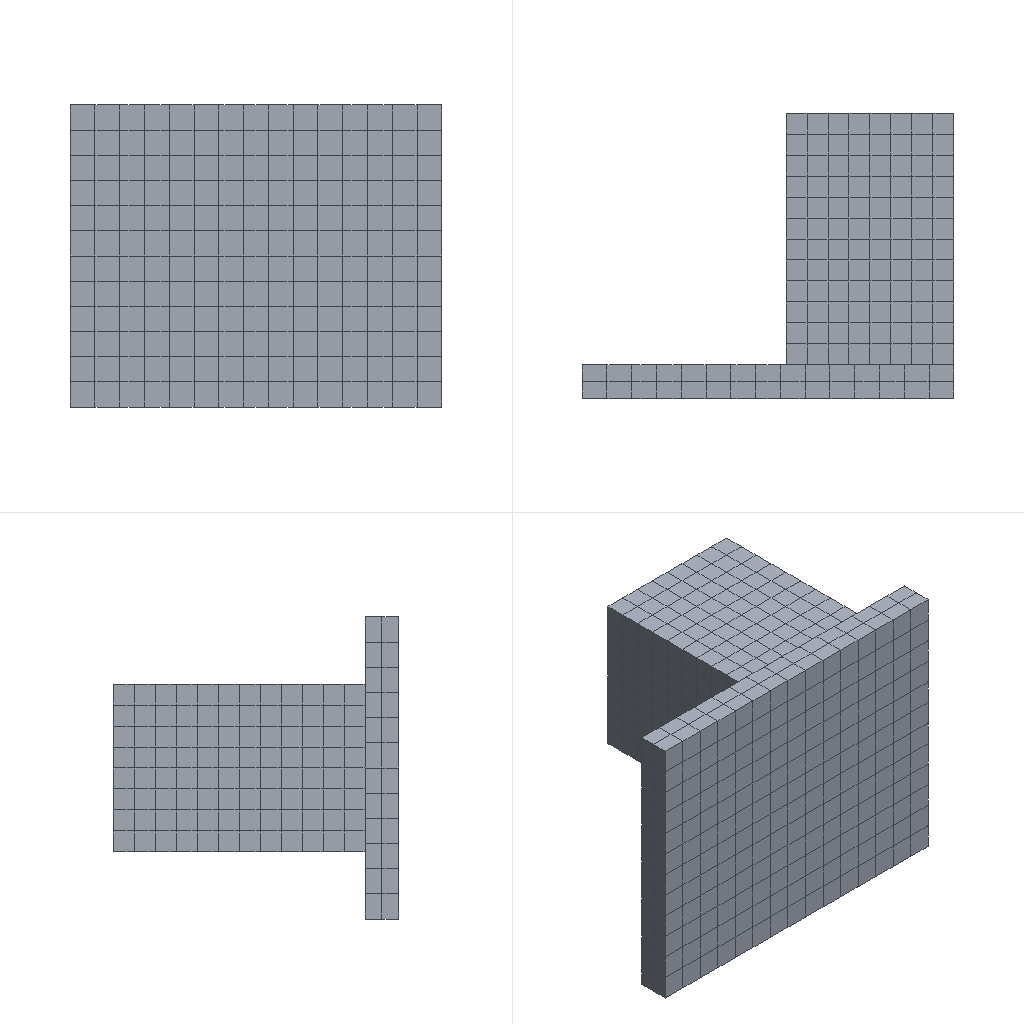Simulation study | ansys workbench
Ansys APDL input file, long lists of numbers shortened:
/batch
/config,noeldb,1     ! force off writing results to database
*get,_wallstrt,active,,time,wall
! ANSYS input file written by Workbench version 2022 R1
! File used for geometry attach:
/title,wbnew--____ (B5)
! ****** Begin Custom Load Command Snippet ******
/COM, ACT Extensions:
/COM,     LSDYNA, 2021.1
/COM,
! ****** End   Custom Load Command Snippet ******
*DIM,_wb_ProjectScratch_dir,string,248
_wb_ProjectScratch_dir(1) = ''
*DIM,_wb_SolverFiles_dir,string,248
_wb_SolverFiles_dir(1) = ''
*DIM,_wb_userfiles_dir,string,248
_wb_userfiles_dir(1) = ''
/com,--- Data in consistent NMM units. See Solving Units in the help system for more information.
/units,MPA
/nopr
/wb,file,start              !  signify a WB generated input file
/prep7
! Turn off shape checking because checks already performed inside WB mesher.
! See help system for more information.
SHPP,OFF,,NOWARN
/nolist
etcon,set             ! allow ANSYS to choose best KEYOP's for 180x elements, resets any applicable keyopt to MAPDL defaults
/com,*********** Nodes for the whole assembly ***********
nblock,3,,6707
(1i9,3e20.9e3)
        1     1.761589892E+00    -5.000000000E-01    -3.750869971E+00
! (6097 more lines like these left out)
-1
/wb,elem,start            !  set before creation of elements
/com,*********** Elements for Body 1 "__2^___1|__-__1" ***********
et,1,186
keyo,1,2,1          ! set full integration on SOLID186
eblock,19,solid,,768
(19i9)
        1        1        1        1        0        0        0        0       20        0      361     2202     3039     3128     3199     2817     3126     3127     3248
! (1535 more lines like these left out)
-1
/com,*********** Elements for Body 2 "__5^___1|__-__1" ***********
et,2,186
keyo,2,2,1          ! set full integration on SOLID186
eblock,19,solid,,360
(19i9)
        2        2        2        2        0        0        0        0       20        0        1        1      573      572      543      308      584      571      570
! (719 more lines like these left out)
-1
/wb,elem,end               !  done creating elements
/com,*********** Send User Defined Coordinate System(s) ***********
csys,0
toffst,273.15,  ! Temperature offset from absolute zero
/com,*********** Set Reference Temperature ***********
tref,22.
/wb,mat,start              !  starting to send materials
/com,*********** Send Materials ***********
Temperature = 'TEMP' ! Temperature
MP,DENS,1,7.85e-09,	! tonne mm^-3
MP,ALPX,1,1.2e-05,	! C^-1
MP,C,1,434000000,	! mm^2 s^-2 C^-1
MP,KXX,1,60.5,	! tonne mm s^-3 C^-1
MP,RSVX,1,0.00017,	! ohm mm
MP,EX,1,200000,	! tonne s^-2 mm^-1
MP,NUXY,1,0.3,
MP,MURX,1,10000,
Temperature = 'TEMP' ! Temperature
MP,DENS,2,7.85e-09,	! tonne mm^-3
MP,ALPX,2,1.2e-05,	! C^-1
MP,C,2,434000000,	! mm^2 s^-2 C^-1
MP,KXX,2,60.5,	! tonne mm s^-3 C^-1
MP,RSVX,2,0.00017,	! ohm mm
MP,EX,2,200000,	! tonne s^-2 mm^-1
MP,NUXY,2,0.3,
MP,MURX,2,10000,
/wb,mat,end                !  done sending materials
!************************* Model Summary ********************
!__2^___1|__-__1,	结构钢,	matid,	1
!__5^___1|__-__1,	结构钢,	matid,	2
!************************* End Model Summary ********************
! get the diagonal of the bounding box. Needed later for other things
*get,_xmin,node,,mnloc,x
*get,_ymin,node,,mnloc,y
*get,_zmin,node,,mnloc,z
*get,_xmax,node,,mxloc,x
*get,_ymax,node,,mxloc,y
*get,_zmax,node,,mxloc,z
_ASMDIAG=(_xmax-_xmin)*(_xmax-_xmin)+(_ymax-_ymin)*(_ymax-_ymin)+(_zmax-_zmin)*(_zmax-_zmin)
_ASMDIAG=SQRT(_ASMDIAG)
/wb,contact,start          !  starting to send contact
/com,*********** Create Contact "接触区域" ***********
/com,            Real Constant Set For Above Contact Is 4 & 3
*set,tid,4
*set,cid,3
r,tid
r,cid
et,tid,170
et,cid,174
eblock,10,,,64
(15i9)
     2109        4        4        4        0     3128     3199     3248     3127     5878     6004     5876     5875
! (63 more lines like these left out)
-1
eblock,10,,,64
(15i9)
     2173        3        3        3        0     3128     3199     3248     3127     5878     6004     5876     5875
! (63 more lines like these left out)
-1
eblock,10,,,56
(15i9)
     2237        3        4        3        0      294      280      586      585     1539     1540     2149     1569
! (55 more lines like these left out)
-1
eblock,10,,,56
(15i9)
     2293        4        3        4        0      294      280      586      585     1539     1540     2149     1569
! (55 more lines like these left out)
-1
keyo,cid,8,2               ! auto create asymmetric contact (from Program Controlled setting)
keyo,cid,10,0              ! adjust contact stiffness each NR iteration (from Program Controlled setting)
keyo,cid,12,5              ! bonded always
keyo,cid,2,0               ! augmented Lagrange
keyo,cid,4,0               ! on Gauss point (from Program Controlled setting)
keyo,cid,9,1               ! ignore initial gaps/penetration
keyo,cid,7,0               ! No Prediction
rmod,tid,3,10.      ! FKN
rmod,tid,5,0.       ! ICONT
rmod,tid,6,0.       ! PINB
rmod,tid,10,0.      ! CNOF
rmod,tid,12,0.      ! FKT
rmod,tid,36,30      ! WB DSID
rmod,cid,3,10.      ! FKN
rmod,cid,5,0.       ! ICONT
rmod,cid,6,0.       ! PINB
rmod,cid,10,0.      ! CNOF
rmod,cid,12,0.      ! FKT
rmod,cid,36,30      ! WB DSID
nsel,all
esel,all
/wb,contact,end            !  done creating contacts
/com,*********** Create Debonding "____" ***********
TB,CZM,3,1,,CBDE
TBDATA,1,1e-07,5e-06,8e-09,5e-06,0.1,0
TBDATA,7,2
*set,matid,3
/golist
/wb,load,start             !  starting to send loads
/com,*********** Fixed Supports ***********
CMBLOCK,_FIXEDSU,NODE,      595
(8i10)
       309       310       311       312       313       314       315       316
! (74 more lines like these left out)
cmsel,s,_FIXEDSU
d,all,all
nsel,all
/com,*********** Define Force Using Surface Effect Elements ***********
local,12,0,0.,0.,0.,0.,0.,0.
csys,0
et,5,154
eblock,10,,,96
(15i9)
     2349        5        5        5       12     3126     3039     3128     3127     5704     5705     5875     5874
! (95 more lines like these left out)
-1
esel,s,type,,5
keyop,5,2,1                ! Apply load in local coordinate system
keyop,5,7,1                ! Use original area so load is constant in large deformation
esel,all
/gst,on,on
fini
*get,_numnode,node,0,count
*get,_numelem,elem,0,count
*get, _MAXELEMNUM, elem, 0, NUM, MAX
*get, _MAXNODENUM, node, 0, NUM, MAX
*get, _MAXELEMTYPE, etyp, 0, NUM, MAX
*get, _MAXREALCONST, real, 0, NUM, MAX
/go
/wb,load,end               !  done creating loads
/com,--- Number of total nodes = %_numnode%
/com,--- Number of contact elements = 336
/com,--- Number of spring elements = 0
/com,--- Number of bearing elements = 0
/com,--- Number of solid elements = 1128
/com,--- Number of condensed parts = 0
/com,--- Number of total elements = %_numelem%
*get,_wallbsol,active,,time,wall
/com,****************************************************************************
/com,*************************    SOLUTION       ********************************
/com,****************************************************************************
/solu
antype,0                   ! static analysis
_thickRatio=0.5     ! Ratio of thick parts in the model
eqsl,sparse,,,,,1
cntr,print,1               ! print out contact info and also make no initial contact an error
dmpoption,emat,no             ! Don't combine emat file for DANSYS
dmpoption,esav,no             ! Don't combine esav file for DANSYS
nldiag,cont,iter           ! print out contact info each equilibrium iteration
rescontrol,define,last,last,,dele	   ! Program Controlled
/com,****************************************************
/com,******************* SOLVE FOR LS 1 OF 1 ****************
esel,s,type,,5
nsle
sfe,all,1,pres,1,133.333
sfe,all,2,pres,1,0.
sfe,all,3,pres,1,-2.31296463463591e-014
nsel,all
esel,all
/nopr
/gopr
autots,on                  ! Workbench Program Controlled automatic time stepping
nsub,5,1000,1              ! due to presence of nonlinear materials
time,1.
outres,erase
outres,all,none
outres,nsol,all,
outres,rsol,all
outres,eangl,all
outres,etmp,all
outres,veng,all
outres,strs,all,
outres,epel,all,
outres,eppl,all,
outres,cont,all,
! *********** WB SOLVE COMMAND ***********
! check interactive state
*get,ANSINTER_,active,,int
*if,ANSINTER_,ne,0,then
/eof
*endif
solve
/com *************** Write FE CONNECTORS *********
CEWRITE,file,ce,,INTE
/com,****************************************************
/com,*************** FINISHED SOLVE FOR LS 1 *************
*get,_wallasol,active,,time,wall
/nopr
*get,_numnode,node,0,count
*get,_numelem,elem,0,count
*get, _MAXELEMNUM, elem, 0, NUM, MAX
*get, _MAXNODENUM, node, 0, NUM, MAX,,,INTERNAL
*get, _MAXELEMTYPE, etyp, 0, NUM, MAX
*get, _MAXREALCONST, real, 0, NUM, MAX
/gopr
/post1
xmlo,ENCODING,ISO-8859-1
xmlo,parm
/xml,parm,xml
fini
/gopr
*get,_walldone,active,,time,wall
_preptime=(_wallbsol-_wallstrt)*3600
_solvtime=(_wallasol-_wallbsol)*3600
_posttime=(_walldone-_wallasol)*3600
_totaltim=(_walldone-_wallstrt)*3600
*get,_dlbratio,active,0,solu,dlbr
*get,_combtime,active,0,solu,comb
*get,_ssmode,active,0,solu,ssmm
*get,_ndofs,active,0,solu,ndof
*get,_sol_end_time,active,0,set,time
*if,_sol_end_time,eq,1.,then
/fclean				!clean distributed files
*endif
/com,--- Total number of nodes = %_numnode%
/com,--- Total number of elements = %_numelem%
/com,--- Element load balance ratio = %_dlbratio%
/com,--- Time to combine distributed files = %_combtime%
/com,--- Sparse memory mode = %_ssmode%
/com,--- Number of DOF = %_ndofs%
/wb,file,end               ! done with WB generated input